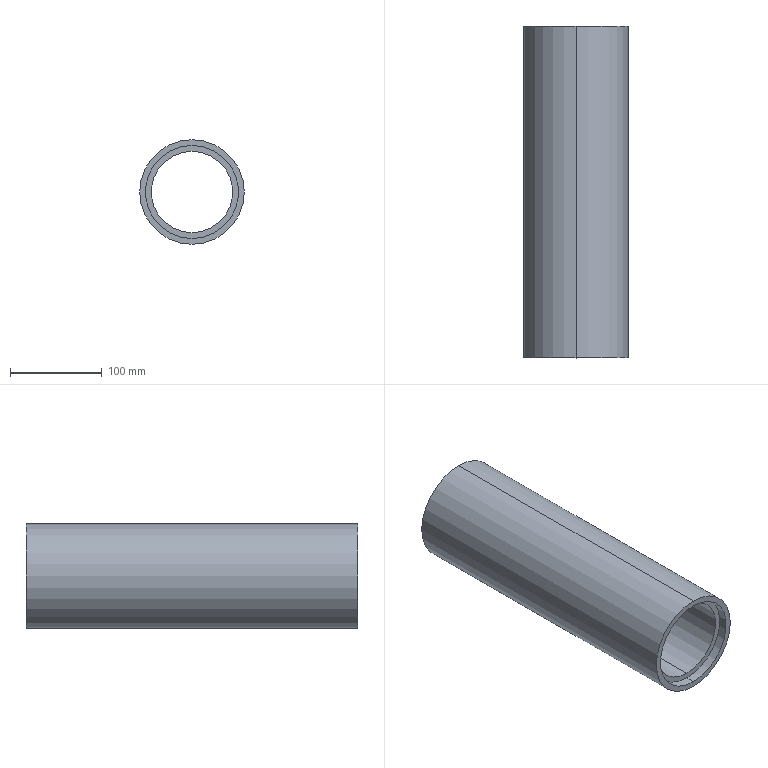Part | STEP file | 1. Barrel | 1 solid | 9 faces | box 114.3 x 362.5 x 114.3 mm | volume 1450450 mm3 | cylinder 6 | plane 3 | commonest cylinder face diameters 88.9 x2 101.6 x2 114.3 x2
STEP:
#1=CARTESIAN_POINT('',(0.,362.5,-57.15));
#2=VERTEX_POINT('',#1);
#3=CARTESIAN_POINT('',(0.,362.5,57.15));
#4=VERTEX_POINT('',#3);
#5=CARTESIAN_POINT('',(0.,362.5,0.));
#6=DIRECTION('',(0.,-1.,0.));
#7=DIRECTION('',(0.,0.,-1.));
#8=AXIS2_PLACEMENT_3D('',#5,#6,#7);
#9=CIRCLE('',#8,57.15);
#10=EDGE_CURVE('',#2,#4,#9,.T.);
#11=ORIENTED_EDGE('',*,*,#10,.T.);
#12=CARTESIAN_POINT('',(0.,0.,57.15));
#13=VERTEX_POINT('',#12);
#14=CARTESIAN_POINT('',(0.,362.5,57.15));
#15=DIRECTION('',(0.,-1.,0.));
#16=VECTOR('',#15,1000.);
#17=LINE('',#14,#16);
#18=EDGE_CURVE('',#4,#13,#17,.T.);
#19=ORIENTED_EDGE('',*,*,#18,.T.);
#20=CARTESIAN_POINT('',(0.,0.,-57.15));
#21=VERTEX_POINT('',#20);
#22=CARTESIAN_POINT('',(0.,0.,0.));
#23=DIRECTION('',(0.,1.,0.));
#24=DIRECTION('',(0.,0.,-1.));
#25=AXIS2_PLACEMENT_3D('',#22,#23,#24);
#26=CIRCLE('',#25,57.15);
#27=EDGE_CURVE('',#13,#21,#26,.T.);
#28=ORIENTED_EDGE('',*,*,#27,.T.);
#29=CARTESIAN_POINT('',(0.,362.5,-57.15));
#30=DIRECTION('',(0.,-1.,0.));
#31=VECTOR('',#30,1000.);
#32=LINE('',#29,#31);
#33=EDGE_CURVE('',#2,#21,#32,.T.);
#34=ORIENTED_EDGE('',*,*,#33,.F.);
#35=EDGE_LOOP('',(#11,#19,#28,#34));
#36=FACE_OUTER_BOUND('',#35,.T.);
#37=CARTESIAN_POINT('',(0.,362.5,0.));
#38=DIRECTION('',(0.,-1.,0.));
#39=DIRECTION('',(0.,0.,-1.));
#40=AXIS2_PLACEMENT_3D('',#37,#38,#39);
#41=CYLINDRICAL_SURFACE('',#40,57.15);
#42=ADVANCED_FACE('',(#36),#41,.T.);
#43=CARTESIAN_POINT('',(0.,10.,50.8));
#44=VERTEX_POINT('',#43);
#45=CARTESIAN_POINT('',(0.,10.,-50.8));
#46=VERTEX_POINT('',#45);
#47=CARTESIAN_POINT('',(0.,10.,0.));
#48=DIRECTION('',(0.,-1.,0.));
#49=DIRECTION('',(0.,0.,-1.));
#50=AXIS2_PLACEMENT_3D('',#47,#48,#49);
#51=CIRCLE('',#50,50.8);
#52=EDGE_CURVE('',#44,#46,#51,.T.);
#53=ORIENTED_EDGE('',*,*,#52,.F.);
#54=CARTESIAN_POINT('',(0.,0.,50.8));
#55=VERTEX_POINT('',#54);
#56=CARTESIAN_POINT('',(0.,10.,50.8));
#57=DIRECTION('',(0.,-1.,0.));
#58=VECTOR('',#57,1000.);
#59=LINE('',#56,#58);
#60=EDGE_CURVE('',#44,#55,#59,.T.);
#61=ORIENTED_EDGE('',*,*,#60,.T.);
#62=CARTESIAN_POINT('',(0.,0.,-50.8));
#63=VERTEX_POINT('',#62);
#64=CARTESIAN_POINT('',(0.,0.,0.));
#65=DIRECTION('',(0.,1.,0.));
#66=DIRECTION('',(0.,0.,-1.));
#67=AXIS2_PLACEMENT_3D('',#64,#65,#66);
#68=CIRCLE('',#67,50.8);
#69=EDGE_CURVE('',#63,#55,#68,.T.);
#70=ORIENTED_EDGE('',*,*,#69,.F.);
#71=CARTESIAN_POINT('',(0.,10.,-50.8));
#72=DIRECTION('',(0.,-1.,0.));
#73=VECTOR('',#72,1000.);
#74=LINE('',#71,#73);
#75=EDGE_CURVE('',#46,#63,#74,.T.);
#76=ORIENTED_EDGE('',*,*,#75,.F.);
#77=EDGE_LOOP('',(#53,#61,#70,#76));
#78=FACE_OUTER_BOUND('',#77,.T.);
#79=CARTESIAN_POINT('',(0.,10.,0.));
#80=DIRECTION('',(0.,-1.,0.));
#81=DIRECTION('',(0.,0.,-1.));
#82=AXIS2_PLACEMENT_3D('',#79,#80,#81);
#83=CYLINDRICAL_SURFACE('',#82,50.8);
#84=ADVANCED_FACE('',(#78),#83,.F.);
#85=CARTESIAN_POINT('',(0.,362.5,-44.45));
#86=VERTEX_POINT('',#85);
#87=CARTESIAN_POINT('',(0.,362.5,44.45));
#88=VERTEX_POINT('',#87);
#89=CARTESIAN_POINT('',(0.,362.5,0.));
#90=DIRECTION('',(0.,1.,0.));
#91=DIRECTION('',(0.,0.,-1.));
#92=AXIS2_PLACEMENT_3D('',#89,#90,#91);
#93=CIRCLE('',#92,44.45);
#94=EDGE_CURVE('',#86,#88,#93,.T.);
#95=ORIENTED_EDGE('',*,*,#94,.T.);
#96=CARTESIAN_POINT('',(0.,10.,44.45));
#97=VERTEX_POINT('',#96);
#98=CARTESIAN_POINT('',(0.,362.5,44.45));
#99=DIRECTION('',(0.,-1.,0.));
#100=VECTOR('',#99,1000.);
#101=LINE('',#98,#100);
#102=EDGE_CURVE('',#88,#97,#101,.T.);
#103=ORIENTED_EDGE('',*,*,#102,.T.);
#104=CARTESIAN_POINT('',(0.,10.,-44.45));
#105=VERTEX_POINT('',#104);
#106=CARTESIAN_POINT('',(0.,10.,0.));
#107=DIRECTION('',(0.,1.,0.));
#108=DIRECTION('',(0.,0.,-1.));
#109=AXIS2_PLACEMENT_3D('',#106,#107,#108);
#110=CIRCLE('',#109,44.45);
#111=EDGE_CURVE('',#105,#97,#110,.T.);
#112=ORIENTED_EDGE('',*,*,#111,.F.);
#113=CARTESIAN_POINT('',(0.,362.5,-44.45));
#114=DIRECTION('',(0.,-1.,0.));
#115=VECTOR('',#114,1000.);
#116=LINE('',#113,#115);
#117=EDGE_CURVE('',#86,#105,#116,.T.);
#118=ORIENTED_EDGE('',*,*,#117,.F.);
#119=EDGE_LOOP('',(#95,#103,#112,#118));
#120=FACE_OUTER_BOUND('',#119,.T.);
#121=CARTESIAN_POINT('',(0.,362.5,0.));
#122=DIRECTION('',(0.,-1.,0.));
#123=DIRECTION('',(0.,0.,-1.));
#124=AXIS2_PLACEMENT_3D('',#121,#122,#123);
#125=CYLINDRICAL_SURFACE('',#124,44.45);
#126=ADVANCED_FACE('',(#120),#125,.F.);
#127=ORIENTED_EDGE('',*,*,#18,.F.);
#128=CARTESIAN_POINT('',(0.,362.5,0.));
#129=DIRECTION('',(0.,-1.,0.));
#130=DIRECTION('',(0.,0.,-1.));
#131=AXIS2_PLACEMENT_3D('',#128,#129,#130);
#132=CIRCLE('',#131,57.15);
#133=EDGE_CURVE('',#4,#2,#132,.T.);
#134=ORIENTED_EDGE('',*,*,#133,.T.);
#135=ORIENTED_EDGE('',*,*,#33,.T.);
#136=CARTESIAN_POINT('',(0.,0.,0.));
#137=DIRECTION('',(0.,1.,0.));
#138=DIRECTION('',(0.,0.,-1.));
#139=AXIS2_PLACEMENT_3D('',#136,#137,#138);
#140=CIRCLE('',#139,57.15);
#141=EDGE_CURVE('',#21,#13,#140,.T.);
#142=ORIENTED_EDGE('',*,*,#141,.T.);
#143=EDGE_LOOP('',(#127,#134,#135,#142));
#144=FACE_OUTER_BOUND('',#143,.T.);
#145=CARTESIAN_POINT('',(0.,362.5,0.));
#146=DIRECTION('',(0.,-1.,0.));
#147=DIRECTION('',(0.,0.,-1.));
#148=AXIS2_PLACEMENT_3D('',#145,#146,#147);
#149=CYLINDRICAL_SURFACE('',#148,57.15);
#150=ADVANCED_FACE('',(#144),#149,.T.);
#151=ORIENTED_EDGE('',*,*,#141,.F.);
#152=ORIENTED_EDGE('',*,*,#27,.F.);
#153=EDGE_LOOP('',(#151,#152));
#154=FACE_OUTER_BOUND('',#153,.T.);
#155=ORIENTED_EDGE('',*,*,#69,.T.);
#156=CARTESIAN_POINT('',(0.,0.,0.));
#157=DIRECTION('',(0.,1.,0.));
#158=DIRECTION('',(0.,0.,-1.));
#159=AXIS2_PLACEMENT_3D('',#156,#157,#158);
#160=CIRCLE('',#159,50.8);
#161=EDGE_CURVE('',#55,#63,#160,.T.);
#162=ORIENTED_EDGE('',*,*,#161,.T.);
#163=EDGE_LOOP('',(#155,#162));
#164=FACE_BOUND('',#163,.T.);
#165=CARTESIAN_POINT('',(0.,0.,0.));
#166=DIRECTION('',(0.,-1.,0.));
#167=DIRECTION('',(0.,0.,-1.));
#168=AXIS2_PLACEMENT_3D('',#165,#166,#167);
#169=PLANE('',#168);
#170=ADVANCED_FACE('',(#154,#164),#169,.T.);
#171=ORIENTED_EDGE('',*,*,#10,.F.);
#172=ORIENTED_EDGE('',*,*,#133,.F.);
#173=EDGE_LOOP('',(#171,#172));
#174=FACE_OUTER_BOUND('',#173,.T.);
#175=ORIENTED_EDGE('',*,*,#94,.F.);
#176=CARTESIAN_POINT('',(0.,362.5,0.));
#177=DIRECTION('',(0.,1.,0.));
#178=DIRECTION('',(0.,0.,-1.));
#179=AXIS2_PLACEMENT_3D('',#176,#177,#178);
#180=CIRCLE('',#179,44.45);
#181=EDGE_CURVE('',#88,#86,#180,.T.);
#182=ORIENTED_EDGE('',*,*,#181,.F.);
#183=EDGE_LOOP('',(#175,#182));
#184=FACE_BOUND('',#183,.T.);
#185=CARTESIAN_POINT('',(0.,362.5,0.));
#186=DIRECTION('',(0.,-1.,0.));
#187=DIRECTION('',(0.,0.,-1.));
#188=AXIS2_PLACEMENT_3D('',#185,#186,#187);
#189=PLANE('',#188);
#190=ADVANCED_FACE('',(#174,#184),#189,.F.);
#191=ORIENTED_EDGE('',*,*,#60,.F.);
#192=CARTESIAN_POINT('',(0.,10.,0.));
#193=DIRECTION('',(0.,-1.,0.));
#194=DIRECTION('',(0.,0.,-1.));
#195=AXIS2_PLACEMENT_3D('',#192,#193,#194);
#196=CIRCLE('',#195,50.8);
#197=EDGE_CURVE('',#46,#44,#196,.T.);
#198=ORIENTED_EDGE('',*,*,#197,.F.);
#199=ORIENTED_EDGE('',*,*,#75,.T.);
#200=ORIENTED_EDGE('',*,*,#161,.F.);
#201=EDGE_LOOP('',(#191,#198,#199,#200));
#202=FACE_OUTER_BOUND('',#201,.T.);
#203=CARTESIAN_POINT('',(0.,10.,0.));
#204=DIRECTION('',(0.,-1.,0.));
#205=DIRECTION('',(0.,0.,-1.));
#206=AXIS2_PLACEMENT_3D('',#203,#204,#205);
#207=CYLINDRICAL_SURFACE('',#206,50.8);
#208=ADVANCED_FACE('',(#202),#207,.F.);
#209=ORIENTED_EDGE('',*,*,#102,.F.);
#210=ORIENTED_EDGE('',*,*,#181,.T.);
#211=ORIENTED_EDGE('',*,*,#117,.T.);
#212=CARTESIAN_POINT('',(0.,10.,0.));
#213=DIRECTION('',(0.,1.,0.));
#214=DIRECTION('',(0.,0.,-1.));
#215=AXIS2_PLACEMENT_3D('',#212,#213,#214);
#216=CIRCLE('',#215,44.45);
#217=EDGE_CURVE('',#97,#105,#216,.T.);
#218=ORIENTED_EDGE('',*,*,#217,.F.);
#219=EDGE_LOOP('',(#209,#210,#211,#218));
#220=FACE_OUTER_BOUND('',#219,.T.);
#221=CARTESIAN_POINT('',(0.,362.5,0.));
#222=DIRECTION('',(0.,-1.,0.));
#223=DIRECTION('',(0.,0.,-1.));
#224=AXIS2_PLACEMENT_3D('',#221,#222,#223);
#225=CYLINDRICAL_SURFACE('',#224,44.45);
#226=ADVANCED_FACE('',(#220),#225,.F.);
#227=ORIENTED_EDGE('',*,*,#197,.T.);
#228=ORIENTED_EDGE('',*,*,#52,.T.);
#229=EDGE_LOOP('',(#227,#228));
#230=FACE_OUTER_BOUND('',#229,.T.);
#231=ORIENTED_EDGE('',*,*,#111,.T.);
#232=ORIENTED_EDGE('',*,*,#217,.T.);
#233=EDGE_LOOP('',(#231,#232));
#234=FACE_BOUND('',#233,.T.);
#235=CARTESIAN_POINT('',(0.,10.,0.));
#236=DIRECTION('',(0.,1.,0.));
#237=DIRECTION('',(0.,0.,1.));
#238=AXIS2_PLACEMENT_3D('',#235,#236,#237);
#239=PLANE('',#238);
#240=ADVANCED_FACE('',(#230,#234),#239,.F.);
#241=CLOSED_SHELL('',(#42,#84,#126,#150,#170,#190,#208,#226,#240));
#242=MANIFOLD_SOLID_BREP('',#241);
#243=CARTESIAN_POINT('',(0.,0.,0.));
#244=DIRECTION('',(0.,0.,1.));
#245=DIRECTION('',(1.,0.,0.));
#246=AXIS2_PLACEMENT_3D('',#243,#244,#245);
#247=(LENGTH_UNIT()NAMED_UNIT(*)SI_UNIT(.MILLI.,.METRE.));
#248=UNCERTAINTY_MEASURE_WITH_UNIT(LENGTH_MEASURE(0.00001),#247,'','');
#249=(NAMED_UNIT(*)PLANE_ANGLE_UNIT()SI_UNIT($,.RADIAN.));
#250=(NAMED_UNIT(*)SI_UNIT($,.STERADIAN.)SOLID_ANGLE_UNIT());
#251=(GEOMETRIC_REPRESENTATION_CONTEXT(3)GLOBAL_UNCERTAINTY_ASSIGNED_CONTEXT((#248))GLOBAL_UNIT_ASSIGNED_CONTEXT((#247,#249,#250))REPRESENTATION_CONTEXT('',''));
#252=ADVANCED_BREP_SHAPE_REPRESENTATION('',(#242,#246),#251);